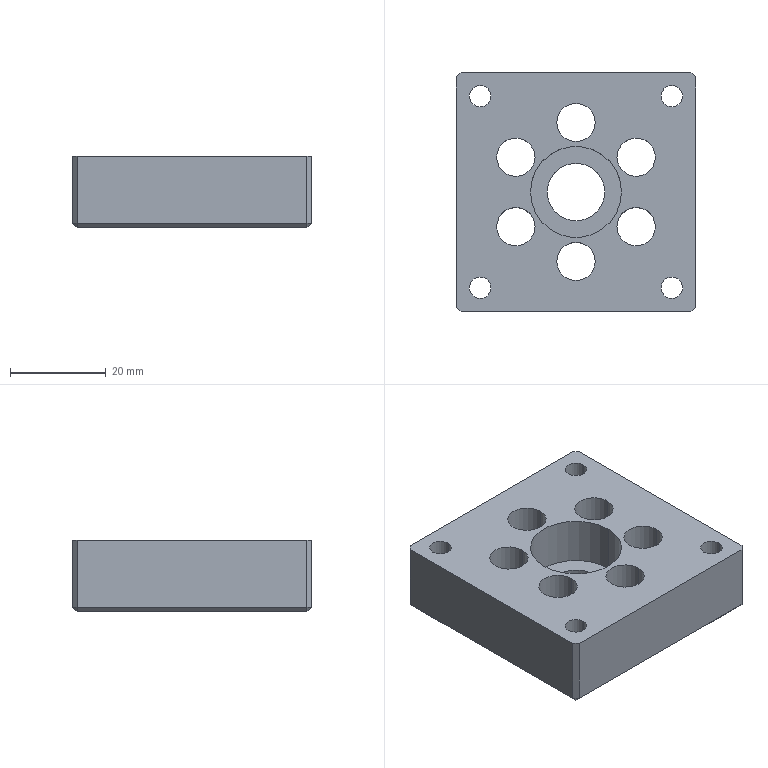Part | STEP file | 04-10 bearing mounting seat | 1 solid | 59 faces | box 50 x 50 x 15 mm | volume 27889 mm3 | cylinder 32 | plane 27 | commonest cylinder face diameters 8 x20 4.5 x8 12 x2 19 x2